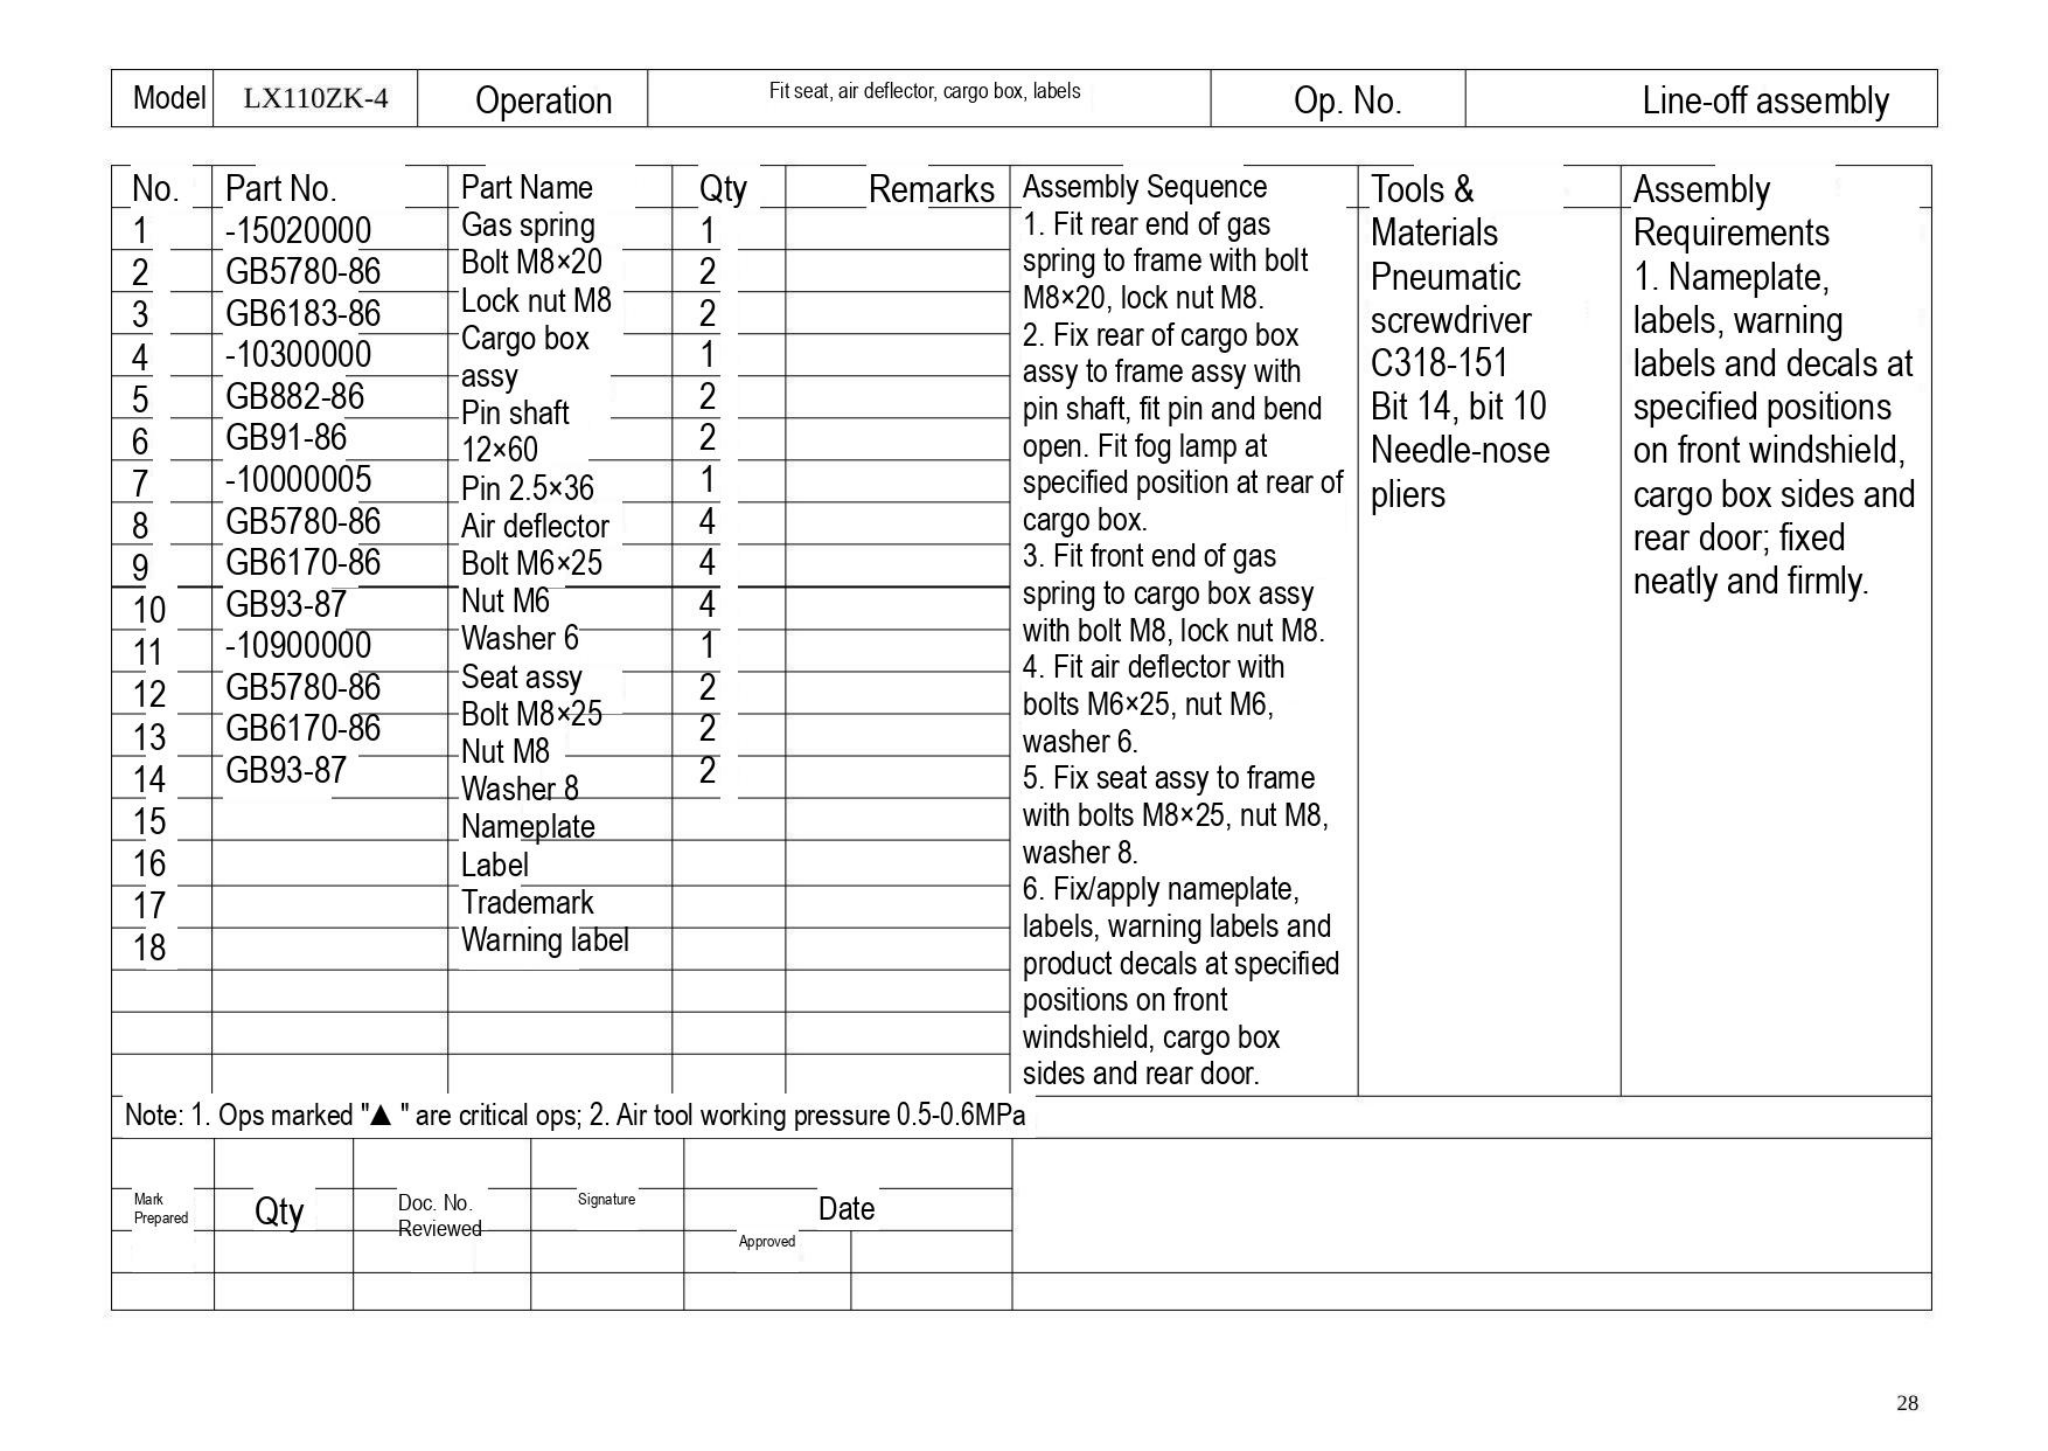| Model | LX110ZK-4 | Operation | Fit seat, air deflector, cargo box, labels | Op. No. | Line-off assembly |
|---|---|---|---|---|---|

| No. | Part No. | Part Name | Qty | Remarks |
|---|---|---|---|---|
| 1 | -15020000 | Gas spring | 1 | |
| 2 | GB5780-86 | Bolt M8×20 | 2 | |
| 3 | GB6183-86 | Lock nut M8 | 2 | |
| 4 | -10300000 | Cargo box assy | 1 | |
| 5 | GB882-86 | Pin shaft 12×60 | 2 | |
| 6 | GB91-86 | Pin 2.5×36 | 2 | |
| 7 | -10000005 | Air deflector | 1 | |
| 8 | GB5780-86 | Bolt M6×25 | 4 | |
| 9 | GB6170-86 | Nut M6 | 4 | |
| 10 | GB93-87 | Washer 6 | 4 | |
| 11 | -10900000 | Seat assy | 1 | |
| 12 | GB5780-86 | Bolt M8×25 | 2 | |
| 13 | GB6170-86 | Nut M8 | 2 | |
| 14 | GB93-87 | Washer 8 | 2 | |
| 15 | | Nameplate | | |
| 16 | | Label | | |
| 17 | | Trademark | | |
| 18 | | Warning label | | |

**Assembly Sequence**
1. Fit rear end of gas spring to frame with bolt M8×20, lock nut M8.
2. Fix rear of cargo box assy to frame assy with pin shaft, fit pin and bend open. Fit fog lamp at specified position at rear of cargo box.
3. Fit front end of gas spring to cargo box assy with bolt M8, lock nut M8.
4. Fit air deflector with bolts M6×25, nut M6, washer 6.
5. Fix seat assy to frame with bolts M8×25, nut M8, washer 8.
6. Fix/apply nameplate, labels, warning labels and product decals at specified positions on front windshield, cargo box sides and rear door.

**Tools & Materials**
Pneumatic screwdriver C318-151
Bit 14, bit 10
Needle-nose pliers

**Assembly Requirements**
1. Nameplate, labels, warning labels and decals at specified positions on front windshield, cargo box sides and rear door; fixed neatly and firmly.

Note: 1. Ops marked "▲ " are critical ops; 2. Air tool working pressure 0.5-0.6MPa

| Mark Prepared | Qty | Doc. No. Reviewed | Signature | Approved | Date |
|---|---|---|---|---|---|
| | | | | | |

28